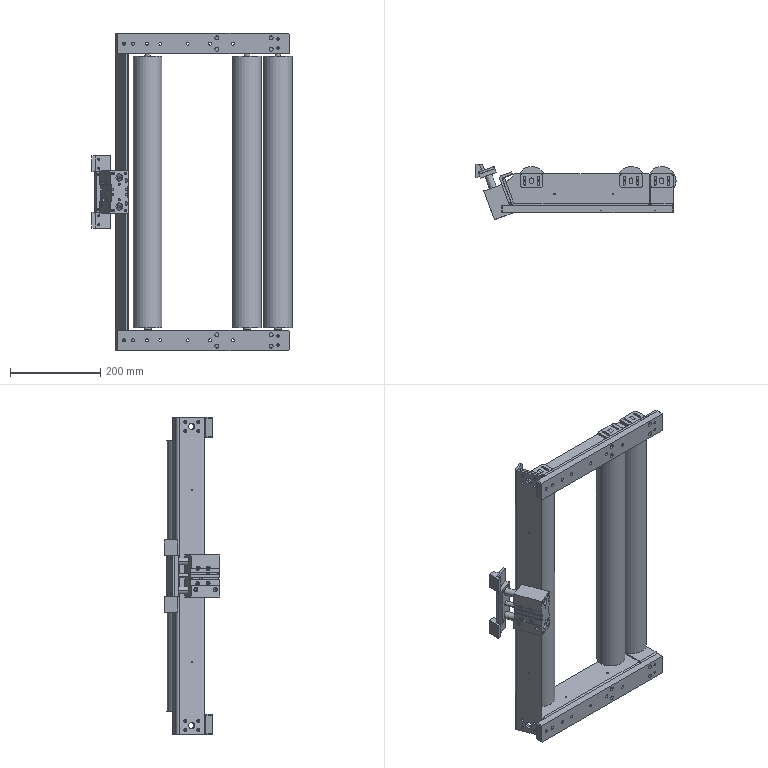Part | SolidWorks | 25 solids | 872 faces | box 442.818 x 122.466 x 702 mm | volume 7134596 mm3 | cylinder 425 | plane 377 | cone 68 | spline 2 | commonest cylinder face diameters 3.3 x36 4.5 x36 10 x36 12 x30 6.8 x28 4.917 x24